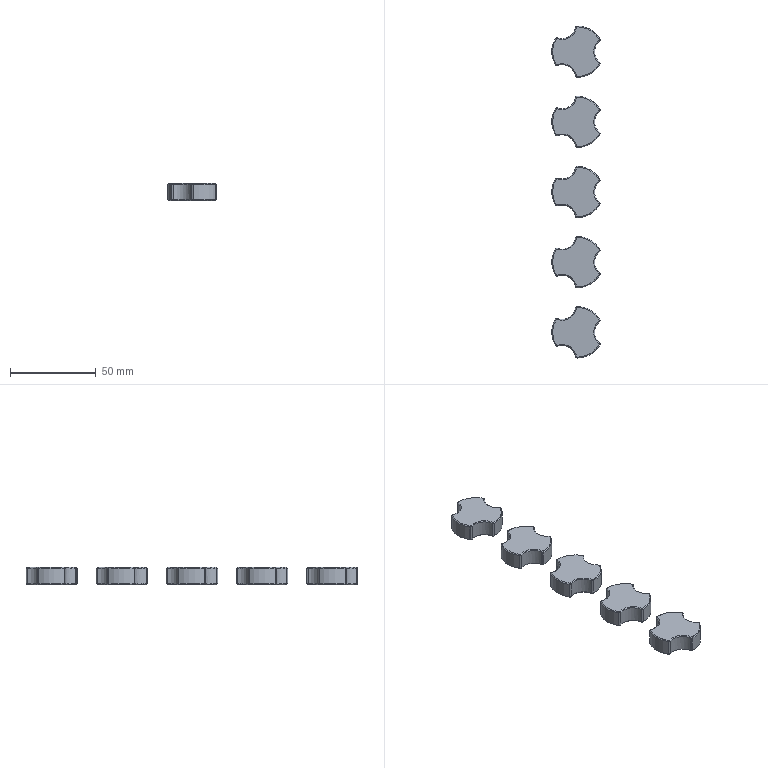NC program | NX | posted with a generic post | part box 28.194 x 194 x 10 mm
Whole program:
N10 G17 G21 G94 G90
(FLOOR_WALL_COPY , TOOL : D80)
N12 T19 M6
N14 G54
N16 G17 G0 G90 X-142. Y0. S6500 M3
N18 G43 Z30. H19
N20 Z7.5
N22 G94 G1 Z4.5 F1500.
N24 X-137.
N26 X137.
N28 X142.
N30 Z7.5
N32 G0 Z30.
N34 X-142.
N36 Z7.
N38 G1 Z4.
N40 X-137.
N42 X137.
N44 X142.
N46 Z7.
N48 G0 Z30.
N50 X-142.
N52 Z6.5
N54 G1 Z3.5
N56 X-137.
N58 X137.
N60 X142.
N62 Z6.5
N64 G0 Z30.
N66 X-142.
N68 Z6.
N70 G1 Z3.
N72 X-137.
N74 X137.
N76 X142.
N78 Z6.
N80 G0 Z30.
N82 X-142.
N84 Z5.5
N86 G1 Z2.5
N88 X-137.
N90 X137.
N92 X142.
N94 Z5.5
N96 G0 Z30.
N98 X-142.
N100 Z5.
N102 G1 Z2.
N104 X-137.
N106 X137.
N108 X142.
N110 Z5.
N112 G0 Z30.
N114 X-142.
N116 Z4.5
N118 G1 Z1.5
N120 X-137.
N122 X137.
N124 X142.
N126 Z4.5
N128 G0 Z30.
N130 X-142.
N132 Z4.
N134 G1 Z1.
N136 X-137.
N138 X137.
N140 X142.
N142 Z4.
N144 G0 Z30.
N146 X-142.
N148 Z3.5
N150 G1 Z0.5
N152 X-137.
N154 X137.
N156 X142.
N158 Z3.5
N160 G0 Z30.
N162 X-142.
N164 Z3.
N166 G1 Z0.
N168 X-137.
N170 X137.
N172 X142.
N174 Z3.
N176 G0 Z30.
N178 M5
(PLANAR_MILL_COPY_COPY_COPY_COPY_COPY , TOOL : D6A45)
N180 T01 M6
N182 G54
N184 G17 G0 G90 X72.93 Y12.908 S9500 M3
N186 G43 Z30. H1
N188 Z0.
N190 G94 G1 Z-1.5 F1250.
N192 G3 X73.93 Y12.913 R1.
N194 G1 X74. Y12.954
N196 G2 X90.14 Y12.872 R16.
N198 X91.004 Y10.472 R2.
N200 G3 X96.352 Y1.207 R7.
N202 G2 X97.999 Y-0.741 R2.
N204 X89.86 Y-14.839 R16.
N206 X87.349 Y-14.387 R2.
N208 G3 X76.651 Y-14.387 R7.
N210 G2 X74.14 Y-14.839 R2.
N212 X66.001 Y-0.741 R16.
N214 X67.648 Y1.207 R2.
N216 G3 X72.996 Y10.472 R7.
N218 G2 X73.93 Y12.913 R2.001
N220 G3 X74.426 Y13.782 R1.
N222 G1 Z0.
N224 G0 Z30.
N226 X31.93 Y12.908
N228 Z0.
N230 G1 Z-1.5
N232 G3 X32.93 Y12.913 R1.
N234 G1 X33. Y12.954
N236 G2 X49.14 Y12.872 R16.
N238 X50.004 Y10.472 R2.
N240 G3 X55.352 Y1.207 R7.
N242 G2 X56.999 Y-0.741 R2.
N244 X48.86 Y-14.839 R16.
N246 X46.349 Y-14.387 R2.
N248 G3 X35.651 Y-14.387 R7.
N250 G2 X33.14 Y-14.839 R2.
N252 X25.001 Y-0.741 R16.
N254 X26.648 Y1.207 R2.
N256 G3 X31.996 Y10.472 R7.
N258 G2 X32.93 Y12.913 R2.001
N260 G3 X33.426 Y13.782 R1.
N262 G1 Z0.
N264 G0 Z30.
N266 X-9.07 Y12.908
N268 Z0.
N270 G1 Z-1.5
N272 G3 X-8.07 Y12.913 R1.
N274 G1 X-8. Y12.954
N276 G2 X8.14 Y12.872 R16.
N278 X9.004 Y10.472 R2.
N280 G3 X14.352 Y1.207 R7.
N282 G2 X15.999 Y-0.741 R2.
N284 X7.86 Y-14.839 R16.
N286 X5.349 Y-14.387 R2.
N288 G3 X-5.349 Y-14.387 R7.
N290 G2 X-7.86 Y-14.839 R2.
N292 X-15.999 Y-0.741 R16.
N294 X-14.352 Y1.207 R2.
N296 G3 X-9.004 Y10.472 R7.
N298 G2 X-8.07 Y12.913 R2.001
N300 G3 X-7.574 Y13.782 R1.
N302 G1 Z0.
N304 G0 Z30.
N306 X-50.07 Y12.908
N308 Z0.
N310 G1 Z-1.5
N312 G3 X-49.07 Y12.913 R1.
N314 G1 X-49. Y12.954
N316 G2 X-32.86 Y12.872 R16.
N318 X-31.996 Y10.472 R2.
N320 G3 X-26.648 Y1.207 R7.
N322 G2 X-25.001 Y-0.741 R2.
N324 X-33.14 Y-14.839 R16.
N326 X-35.651 Y-14.387 R2.
N328 G3 X-46.349 Y-14.387 R7.
N330 G2 X-48.86 Y-14.839 R2.
N332 X-56.999 Y-0.741 R16.
N334 X-55.352 Y1.207 R2.
N336 G3 X-50.004 Y10.472 R7.
N338 G2 X-49.07 Y12.913 R2.001
N340 G3 X-48.574 Y13.782 R1.
N342 G1 Z0.
N344 G0 Z30.
N346 X-91.07 Y12.908
N348 Z0.
N350 G1 Z-1.5
N352 G3 X-90.07 Y12.913 R1.
N354 G1 X-90. Y12.954
N356 G2 X-73.86 Y12.872 R16.
N358 X-72.996 Y10.472 R2.
N360 G3 X-67.648 Y1.207 R7.
N362 G2 X-66.001 Y-0.741 R2.
N364 X-74.14 Y-14.839 R16.
N366 X-76.651 Y-14.387 R2.
N368 G3 X-87.349 Y-14.387 R7.
N370 G2 X-89.86 Y-14.839 R2.
N372 X-97.999 Y-0.741 R16.
N374 X-96.352 Y1.207 R2.
N376 G3 X-91.004 Y10.472 R7.
N378 G2 X-90.07 Y12.913 R2.001
N380 G3 X-89.574 Y13.782 R1.
N382 G1 Z0.
N384 G0 Z30.
N386 M5
N388 M2